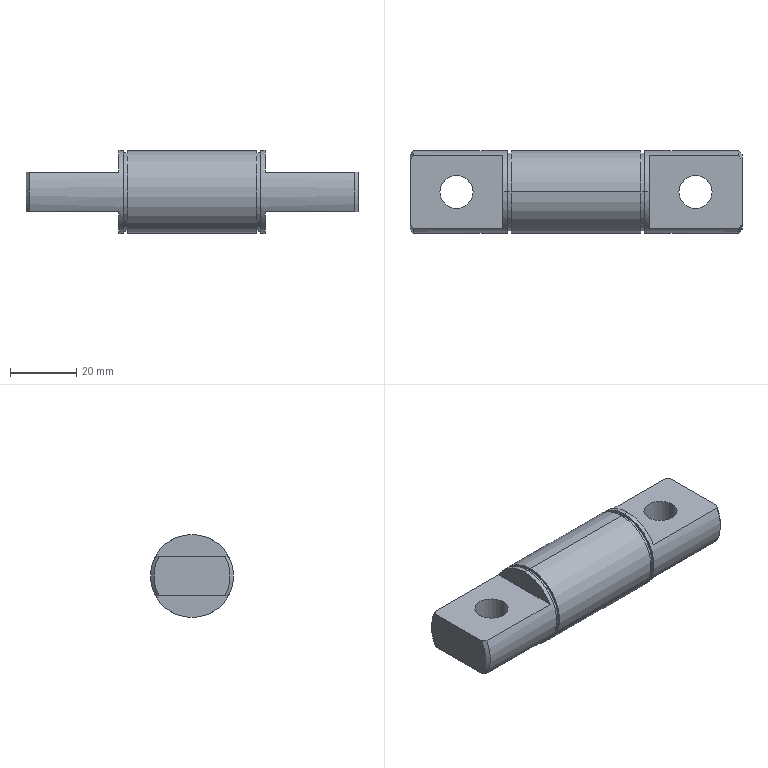Part | STEP file | tension shaft_SUS304 | 1 solid | 32 faces | box 100 x 25 x 25 mm | volume 35682 mm3 | cylinder 14 | plane 14 | cone 4 | commonest cylinder face diameters 25 x6 10 x4 23.5 x4